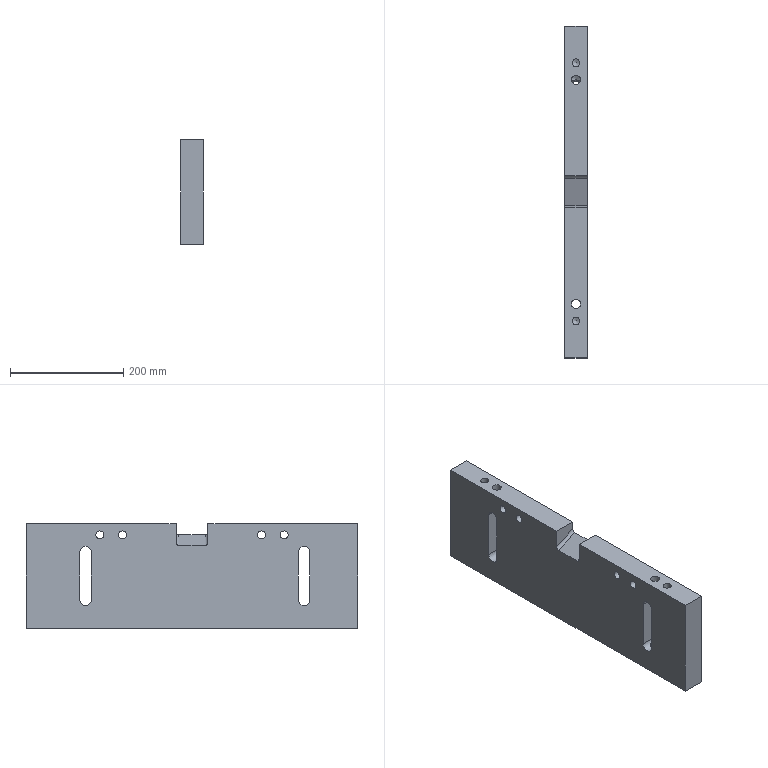Part | STEP file | 1 solid | 39 faces | box 40 x 585 x 185 mm | volume 4012325 mm3 | cylinder 19 | plane 14 | cone 6 | commonest cylinder face diameters 14 x9 16 x4 20 x4 10 x2
STEP:
#1=CARTESIAN_POINT('',(350.,-207.5,-242.));
#2=VERTEX_POINT('',#1);
#3=CARTESIAN_POINT('',(350.,-187.5,-242.));
#4=VERTEX_POINT('',#3);
#5=CARTESIAN_POINT('',(350.,-197.5,-242.));
#6=DIRECTION('',(1.,0.,0.));
#7=DIRECTION('',(0.,0.,-1.));
#8=AXIS2_PLACEMENT_3D('',#5,#6,#7);
#9=CIRCLE('',#8,10.);
#10=EDGE_CURVE('',#2,#4,#9,.T.);
#11=ORIENTED_EDGE('',*,*,#10,.F.);
#12=CARTESIAN_POINT('',(350.,-207.5,-157.));
#13=VERTEX_POINT('',#12);
#14=CARTESIAN_POINT('',(350.,-207.5,-292.));
#15=DIRECTION('',(0.,0.,1.));
#16=VECTOR('',#15,1.);
#17=LINE('',#14,#16);
#18=EDGE_CURVE('',#2,#13,#17,.T.);
#19=ORIENTED_EDGE('',*,*,#18,.T.);
#20=CARTESIAN_POINT('',(350.,-187.5,-157.));
#21=VERTEX_POINT('',#20);
#22=CARTESIAN_POINT('',(350.,-197.5,-157.));
#23=DIRECTION('',(1.,0.,0.));
#24=DIRECTION('',(0.,0.,-1.));
#25=AXIS2_PLACEMENT_3D('',#22,#23,#24);
#26=CIRCLE('',#25,10.);
#27=EDGE_CURVE('',#21,#13,#26,.T.);
#28=ORIENTED_EDGE('',*,*,#27,.F.);
#29=CARTESIAN_POINT('',(350.,-187.5,-107.));
#30=DIRECTION('',(0.,0.,1.));
#31=VECTOR('',#30,1.);
#32=LINE('',#29,#31);
#33=EDGE_CURVE('',#4,#21,#32,.T.);
#34=ORIENTED_EDGE('',*,*,#33,.F.);
#35=EDGE_LOOP('',(#11,#19,#28,#34));
#36=FACE_BOUND('',#35,.T.);
#37=CARTESIAN_POINT('',(350.,28.14,-121.483));
#38=VERTEX_POINT('',#37);
#39=CARTESIAN_POINT('',(350.,28.14,-107.));
#40=VERTEX_POINT('',#39);
#41=CARTESIAN_POINT('',(350.,28.14,-107.));
#42=DIRECTION('',(0.,0.,1.));
#43=VECTOR('',#42,1.);
#44=LINE('',#41,#43);
#45=EDGE_CURVE('',#38,#40,#44,.T.);
#46=ORIENTED_EDGE('',*,*,#45,.F.);
#47=CARTESIAN_POINT('',(350.,23.14,-127.));
#48=VERTEX_POINT('',#47);
#49=CARTESIAN_POINT('',(350.,23.14,-121.483));
#50=DIRECTION('',(-1.,0.,0.));
#51=DIRECTION('',(0.,0.,-1.));
#52=AXIS2_PLACEMENT_3D('',#49,#50,#51);
#53=ELLIPSE('',#52,5.517,5.);
#54=EDGE_CURVE('',#38,#48,#53,.T.);
#55=ORIENTED_EDGE('',*,*,#54,.T.);
#56=CARTESIAN_POINT('',(350.,-23.14,-127.));
#57=VERTEX_POINT('',#56);
#58=CARTESIAN_POINT('',(350.,-1.,-127.));
#59=DIRECTION('',(0.,1.,0.));
#60=VECTOR('',#59,1.);
#61=LINE('',#58,#60);
#62=EDGE_CURVE('',#57,#48,#61,.T.);
#63=ORIENTED_EDGE('',*,*,#62,.F.);
#64=CARTESIAN_POINT('',(350.,-28.14,-121.483));
#65=VERTEX_POINT('',#64);
#66=CARTESIAN_POINT('',(350.,-23.14,-121.483));
#67=DIRECTION('',(-1.,0.,0.));
#68=DIRECTION('',(0.,0.,1.));
#69=AXIS2_PLACEMENT_3D('',#66,#67,#68);
#70=ELLIPSE('',#69,5.517,5.);
#71=EDGE_CURVE('',#57,#65,#70,.T.);
#72=ORIENTED_EDGE('',*,*,#71,.T.);
#73=CARTESIAN_POINT('',(350.,-28.14,-107.));
#74=VERTEX_POINT('',#73);
#75=CARTESIAN_POINT('',(350.,-28.14,-107.));
#76=DIRECTION('',(0.,0.,1.));
#77=VECTOR('',#76,1.);
#78=LINE('',#75,#77);
#79=EDGE_CURVE('',#65,#74,#78,.T.);
#80=ORIENTED_EDGE('',*,*,#79,.T.);
#81=CARTESIAN_POINT('',(350.,-292.5,-107.));
#82=VERTEX_POINT('',#81);
#83=CARTESIAN_POINT('',(350.,-1.,-107.));
#84=DIRECTION('',(0.,-1.,0.));
#85=VECTOR('',#84,1.);
#86=LINE('',#83,#85);
#87=EDGE_CURVE('',#74,#82,#86,.T.);
#88=ORIENTED_EDGE('',*,*,#87,.T.);
#89=CARTESIAN_POINT('',(350.,-292.5,-292.));
#90=VERTEX_POINT('',#89);
#91=CARTESIAN_POINT('',(350.,-292.5,-107.));
#92=DIRECTION('',(0.,0.,1.));
#93=VECTOR('',#92,1.);
#94=LINE('',#91,#93);
#95=EDGE_CURVE('',#90,#82,#94,.T.);
#96=ORIENTED_EDGE('',*,*,#95,.F.);
#97=CARTESIAN_POINT('',(350.,292.5,-292.));
#98=VERTEX_POINT('',#97);
#99=CARTESIAN_POINT('',(350.,-1.,-292.));
#100=DIRECTION('',(0.,-1.,0.));
#101=VECTOR('',#100,1.);
#102=LINE('',#99,#101);
#103=EDGE_CURVE('',#98,#90,#102,.T.);
#104=ORIENTED_EDGE('',*,*,#103,.F.);
#105=CARTESIAN_POINT('',(350.,292.5,-107.));
#106=VERTEX_POINT('',#105);
#107=CARTESIAN_POINT('',(350.,292.5,-107.));
#108=DIRECTION('',(0.,0.,1.));
#109=VECTOR('',#108,1.);
#110=LINE('',#107,#109);
#111=EDGE_CURVE('',#98,#106,#110,.T.);
#112=ORIENTED_EDGE('',*,*,#111,.T.);
#113=CARTESIAN_POINT('',(350.,-1.,-107.));
#114=DIRECTION('',(0.,-1.,0.));
#115=VECTOR('',#114,1.);
#116=LINE('',#113,#115);
#117=EDGE_CURVE('',#106,#40,#116,.T.);
#118=ORIENTED_EDGE('',*,*,#117,.T.);
#119=EDGE_LOOP('',(#46,#55,#63,#72,#80,#88,#96,#104,#112,#118));
#120=FACE_BOUND('',#119,.T.);
#121=CARTESIAN_POINT('',(350.,-162.5,-120.));
#122=VERTEX_POINT('',#121);
#123=CARTESIAN_POINT('',(350.,-162.5,-127.));
#124=DIRECTION('',(-1.,0.,0.));
#125=DIRECTION('',(0.,0.,1.));
#126=AXIS2_PLACEMENT_3D('',#123,#124,#125);
#127=CIRCLE('',#126,7.);
#128=EDGE_CURVE('',#122,#122,#127,.T.);
#129=ORIENTED_EDGE('',*,*,#128,.T.);
#130=EDGE_LOOP('',(#129));
#131=FACE_BOUND('',#130,.T.);
#132=CARTESIAN_POINT('',(350.,-122.5,-120.));
#133=VERTEX_POINT('',#132);
#134=CARTESIAN_POINT('',(350.,-122.5,-127.));
#135=DIRECTION('',(1.,0.,0.));
#136=DIRECTION('',(0.,0.,1.));
#137=AXIS2_PLACEMENT_3D('',#134,#135,#136);
#138=CIRCLE('',#137,7.);
#139=EDGE_CURVE('',#133,#133,#138,.T.);
#140=ORIENTED_EDGE('',*,*,#139,.F.);
#141=EDGE_LOOP('',(#140));
#142=FACE_BOUND('',#141,.T.);
#143=CARTESIAN_POINT('',(350.,162.5,-120.));
#144=VERTEX_POINT('',#143);
#145=CARTESIAN_POINT('',(350.,162.5,-127.));
#146=DIRECTION('',(1.,0.,0.));
#147=DIRECTION('',(0.,0.,1.));
#148=AXIS2_PLACEMENT_3D('',#145,#146,#147);
#149=CIRCLE('',#148,7.);
#150=EDGE_CURVE('',#144,#144,#149,.T.);
#151=ORIENTED_EDGE('',*,*,#150,.F.);
#152=EDGE_LOOP('',(#151));
#153=FACE_BOUND('',#152,.T.);
#154=CARTESIAN_POINT('',(350.,122.5,-120.));
#155=VERTEX_POINT('',#154);
#156=CARTESIAN_POINT('',(350.,122.5,-127.));
#157=DIRECTION('',(-1.,0.,0.));
#158=DIRECTION('',(0.,0.,1.));
#159=AXIS2_PLACEMENT_3D('',#156,#157,#158);
#160=CIRCLE('',#159,7.);
#161=EDGE_CURVE('',#155,#155,#160,.T.);
#162=ORIENTED_EDGE('',*,*,#161,.T.);
#163=EDGE_LOOP('',(#162));
#164=FACE_BOUND('',#163,.T.);
#165=CARTESIAN_POINT('',(350.,177.5,-242.));
#166=VERTEX_POINT('',#165);
#167=CARTESIAN_POINT('',(350.,197.5,-242.));
#168=VERTEX_POINT('',#167);
#169=CARTESIAN_POINT('',(350.,187.5,-242.));
#170=DIRECTION('',(1.,0.,0.));
#171=DIRECTION('',(0.,0.,-1.));
#172=AXIS2_PLACEMENT_3D('',#169,#170,#171);
#173=CIRCLE('',#172,10.);
#174=EDGE_CURVE('',#166,#168,#173,.T.);
#175=ORIENTED_EDGE('',*,*,#174,.F.);
#176=CARTESIAN_POINT('',(350.,177.5,-157.));
#177=VERTEX_POINT('',#176);
#178=CARTESIAN_POINT('',(350.,177.5,-292.));
#179=DIRECTION('',(0.,0.,1.));
#180=VECTOR('',#179,1.);
#181=LINE('',#178,#180);
#182=EDGE_CURVE('',#166,#177,#181,.T.);
#183=ORIENTED_EDGE('',*,*,#182,.T.);
#184=CARTESIAN_POINT('',(350.,197.5,-157.));
#185=VERTEX_POINT('',#184);
#186=CARTESIAN_POINT('',(350.,187.5,-157.));
#187=DIRECTION('',(1.,0.,0.));
#188=DIRECTION('',(0.,0.,-1.));
#189=AXIS2_PLACEMENT_3D('',#186,#187,#188);
#190=CIRCLE('',#189,10.);
#191=EDGE_CURVE('',#185,#177,#190,.T.);
#192=ORIENTED_EDGE('',*,*,#191,.F.);
#193=CARTESIAN_POINT('',(350.,197.5,-107.));
#194=DIRECTION('',(0.,0.,1.));
#195=VECTOR('',#194,1.);
#196=LINE('',#193,#195);
#197=EDGE_CURVE('',#168,#185,#196,.T.);
#198=ORIENTED_EDGE('',*,*,#197,.F.);
#199=EDGE_LOOP('',(#175,#183,#192,#198));
#200=FACE_BOUND('',#199,.T.);
#201=CARTESIAN_POINT('',(350.,-1.,-107.));
#202=DIRECTION('',(1.,0.,0.));
#203=DIRECTION('',(0.,-1.,0.));
#204=AXIS2_PLACEMENT_3D('',#201,#202,#203);
#205=PLANE('',#204);
#206=ADVANCED_FACE('',(#36,#120,#131,#142,#153,#164,#200),#205,.T.);
#207=CARTESIAN_POINT('',(310.,-187.5,-242.));
#208=VERTEX_POINT('',#207);
#209=CARTESIAN_POINT('',(310.,-207.5,-242.));
#210=VERTEX_POINT('',#209);
#211=CARTESIAN_POINT('',(310.,-197.5,-242.));
#212=DIRECTION('',(-1.,0.,0.));
#213=DIRECTION('',(0.,0.,1.));
#214=AXIS2_PLACEMENT_3D('',#211,#212,#213);
#215=CIRCLE('',#214,10.);
#216=EDGE_CURVE('',#208,#210,#215,.T.);
#217=ORIENTED_EDGE('',*,*,#216,.F.);
#218=CARTESIAN_POINT('',(310.,-187.5,-157.));
#219=VERTEX_POINT('',#218);
#220=CARTESIAN_POINT('',(310.,-187.5,-292.));
#221=DIRECTION('',(0.,0.,1.));
#222=VECTOR('',#221,1.);
#223=LINE('',#220,#222);
#224=EDGE_CURVE('',#208,#219,#223,.T.);
#225=ORIENTED_EDGE('',*,*,#224,.T.);
#226=CARTESIAN_POINT('',(310.,-207.5,-157.));
#227=VERTEX_POINT('',#226);
#228=CARTESIAN_POINT('',(310.,-197.5,-157.));
#229=DIRECTION('',(-1.,0.,0.));
#230=DIRECTION('',(0.,0.,1.));
#231=AXIS2_PLACEMENT_3D('',#228,#229,#230);
#232=CIRCLE('',#231,10.);
#233=EDGE_CURVE('',#227,#219,#232,.T.);
#234=ORIENTED_EDGE('',*,*,#233,.F.);
#235=CARTESIAN_POINT('',(310.,-207.5,-107.));
#236=DIRECTION('',(0.,0.,1.));
#237=VECTOR('',#236,1.);
#238=LINE('',#235,#237);
#239=EDGE_CURVE('',#210,#227,#238,.T.);
#240=ORIENTED_EDGE('',*,*,#239,.F.);
#241=EDGE_LOOP('',(#217,#225,#234,#240));
#242=FACE_BOUND('',#241,.T.);
#243=CARTESIAN_POINT('',(310.,122.5,-120.));
#244=VERTEX_POINT('',#243);
#245=CARTESIAN_POINT('',(310.,122.5,-127.));
#246=DIRECTION('',(-1.,0.,0.));
#247=DIRECTION('',(0.,0.,1.));
#248=AXIS2_PLACEMENT_3D('',#245,#246,#247);
#249=CIRCLE('',#248,7.);
#250=EDGE_CURVE('',#244,#244,#249,.T.);
#251=ORIENTED_EDGE('',*,*,#250,.F.);
#252=EDGE_LOOP('',(#251));
#253=FACE_BOUND('',#252,.T.);
#254=CARTESIAN_POINT('',(310.,162.5,-120.));
#255=VERTEX_POINT('',#254);
#256=CARTESIAN_POINT('',(310.,162.5,-127.));
#257=DIRECTION('',(1.,0.,0.));
#258=DIRECTION('',(0.,0.,1.));
#259=AXIS2_PLACEMENT_3D('',#256,#257,#258);
#260=CIRCLE('',#259,7.);
#261=EDGE_CURVE('',#255,#255,#260,.T.);
#262=ORIENTED_EDGE('',*,*,#261,.T.);
#263=EDGE_LOOP('',(#262));
#264=FACE_BOUND('',#263,.T.);
#265=CARTESIAN_POINT('',(310.,-122.5,-120.));
#266=VERTEX_POINT('',#265);
#267=CARTESIAN_POINT('',(310.,-122.5,-127.));
#268=DIRECTION('',(1.,0.,0.));
#269=DIRECTION('',(0.,0.,1.));
#270=AXIS2_PLACEMENT_3D('',#267,#268,#269);
#271=CIRCLE('',#270,7.);
#272=EDGE_CURVE('',#266,#266,#271,.T.);
#273=ORIENTED_EDGE('',*,*,#272,.T.);
#274=EDGE_LOOP('',(#273));
#275=FACE_BOUND('',#274,.T.);
#276=CARTESIAN_POINT('',(310.,-162.5,-120.));
#277=VERTEX_POINT('',#276);
#278=CARTESIAN_POINT('',(310.,-162.5,-127.));
#279=DIRECTION('',(-1.,0.,0.));
#280=DIRECTION('',(0.,0.,1.));
#281=AXIS2_PLACEMENT_3D('',#278,#279,#280);
#282=CIRCLE('',#281,7.);
#283=EDGE_CURVE('',#277,#277,#282,.T.);
#284=ORIENTED_EDGE('',*,*,#283,.F.);
#285=EDGE_LOOP('',(#284));
#286=FACE_BOUND('',#285,.T.);
#287=CARTESIAN_POINT('',(310.,-292.5,-107.));
#288=VERTEX_POINT('',#287);
#289=CARTESIAN_POINT('',(310.,-28.14,-107.));
#290=VERTEX_POINT('',#289);
#291=CARTESIAN_POINT('',(310.,-1.,-107.));
#292=DIRECTION('',(0.,1.,0.));
#293=VECTOR('',#292,1.);
#294=LINE('',#291,#293);
#295=EDGE_CURVE('',#288,#290,#294,.T.);
#296=ORIENTED_EDGE('',*,*,#295,.T.);
#297=CARTESIAN_POINT('',(310.,-28.14,-140.135));
#298=VERTEX_POINT('',#297);
#299=CARTESIAN_POINT('',(310.,-28.14,-107.));
#300=DIRECTION('',(0.,0.,-1.));
#301=VECTOR('',#300,1.);
#302=LINE('',#299,#301);
#303=EDGE_CURVE('',#290,#298,#302,.T.);
#304=ORIENTED_EDGE('',*,*,#303,.T.);
#305=CARTESIAN_POINT('',(310.,-23.14,-145.652));
#306=VERTEX_POINT('',#305);
#307=CARTESIAN_POINT('',(310.,-23.14,-140.135));
#308=DIRECTION('',(1.,0.,0.));
#309=DIRECTION('',(0.,0.,1.));
#310=AXIS2_PLACEMENT_3D('',#307,#308,#309);
#311=ELLIPSE('',#310,5.517,5.);
#312=EDGE_CURVE('',#298,#306,#311,.T.);
#313=ORIENTED_EDGE('',*,*,#312,.T.);
#314=CARTESIAN_POINT('',(310.,23.14,-145.652));
#315=VERTEX_POINT('',#314);
#316=CARTESIAN_POINT('',(310.,-1.,-145.652));
#317=DIRECTION('',(0.,1.,0.));
#318=VECTOR('',#317,1.);
#319=LINE('',#316,#318);
#320=EDGE_CURVE('',#306,#315,#319,.T.);
#321=ORIENTED_EDGE('',*,*,#320,.T.);
#322=CARTESIAN_POINT('',(310.,28.14,-140.135));
#323=VERTEX_POINT('',#322);
#324=CARTESIAN_POINT('',(310.,23.14,-140.135));
#325=DIRECTION('',(1.,0.,0.));
#326=DIRECTION('',(0.,0.,-1.));
#327=AXIS2_PLACEMENT_3D('',#324,#325,#326);
#328=ELLIPSE('',#327,5.517,5.);
#329=EDGE_CURVE('',#315,#323,#328,.T.);
#330=ORIENTED_EDGE('',*,*,#329,.T.);
#331=CARTESIAN_POINT('',(310.,28.14,-107.));
#332=VERTEX_POINT('',#331);
#333=CARTESIAN_POINT('',(310.,28.14,-107.));
#334=DIRECTION('',(0.,0.,1.));
#335=VECTOR('',#334,1.);
#336=LINE('',#333,#335);
#337=EDGE_CURVE('',#323,#332,#336,.T.);
#338=ORIENTED_EDGE('',*,*,#337,.T.);
#339=CARTESIAN_POINT('',(310.,292.5,-107.));
#340=VERTEX_POINT('',#339);
#341=CARTESIAN_POINT('',(310.,-1.,-107.));
#342=DIRECTION('',(0.,1.,0.));
#343=VECTOR('',#342,1.);
#344=LINE('',#341,#343);
#345=EDGE_CURVE('',#332,#340,#344,.T.);
#346=ORIENTED_EDGE('',*,*,#345,.T.);
#347=CARTESIAN_POINT('',(310.,292.5,-292.));
#348=VERTEX_POINT('',#347);
#349=CARTESIAN_POINT('',(310.,292.5,-107.));
#350=DIRECTION('',(0.,0.,1.));
#351=VECTOR('',#350,1.);
#352=LINE('',#349,#351);
#353=EDGE_CURVE('',#348,#340,#352,.T.);
#354=ORIENTED_EDGE('',*,*,#353,.F.);
#355=CARTESIAN_POINT('',(310.,-292.5,-292.));
#356=VERTEX_POINT('',#355);
#357=CARTESIAN_POINT('',(310.,-1.,-292.));
#358=DIRECTION('',(0.,1.,0.));
#359=VECTOR('',#358,1.);
#360=LINE('',#357,#359);
#361=EDGE_CURVE('',#356,#348,#360,.T.);
#362=ORIENTED_EDGE('',*,*,#361,.F.);
#363=CARTESIAN_POINT('',(310.,-292.5,-107.));
#364=DIRECTION('',(0.,0.,1.));
#365=VECTOR('',#364,1.);
#366=LINE('',#363,#365);
#367=EDGE_CURVE('',#356,#288,#366,.T.);
#368=ORIENTED_EDGE('',*,*,#367,.T.);
#369=EDGE_LOOP('',(#296,#304,#313,#321,#330,#338,#346,#354,#362,#368));
#370=FACE_BOUND('',#369,.T.);
#371=CARTESIAN_POINT('',(310.,197.5,-242.));
#372=VERTEX_POINT('',#371);
#373=CARTESIAN_POINT('',(310.,177.5,-242.));
#374=VERTEX_POINT('',#373);
#375=CARTESIAN_POINT('',(310.,187.5,-242.));
#376=DIRECTION('',(-1.,0.,0.));
#377=DIRECTION('',(0.,0.,1.));
#378=AXIS2_PLACEMENT_3D('',#375,#376,#377);
#379=CIRCLE('',#378,10.);
#380=EDGE_CURVE('',#372,#374,#379,.T.);
#381=ORIENTED_EDGE('',*,*,#380,.F.);
#382=CARTESIAN_POINT('',(310.,197.5,-157.));
#383=VERTEX_POINT('',#382);
#384=CARTESIAN_POINT('',(310.,197.5,-292.));
#385=DIRECTION('',(0.,0.,1.));
#386=VECTOR('',#385,1.);
#387=LINE('',#384,#386);
#388=EDGE_CURVE('',#372,#383,#387,.T.);
#389=ORIENTED_EDGE('',*,*,#388,.T.);
#390=CARTESIAN_POINT('',(310.,177.5,-157.));
#391=VERTEX_POINT('',#390);
#392=CARTESIAN_POINT('',(310.,187.5,-157.));
#393=DIRECTION('',(-1.,0.,0.));
#394=DIRECTION('',(0.,0.,1.));
#395=AXIS2_PLACEMENT_3D('',#392,#393,#394);
#396=CIRCLE('',#395,10.);
#397=EDGE_CURVE('',#391,#383,#396,.T.);
#398=ORIENTED_EDGE('',*,*,#397,.F.);
#399=CARTESIAN_POINT('',(310.,177.5,-107.));
#400=DIRECTION('',(0.,0.,1.));
#401=VECTOR('',#400,1.);
#402=LINE('',#399,#401);
#403=EDGE_CURVE('',#374,#391,#402,.T.);
#404=ORIENTED_EDGE('',*,*,#403,.F.);
#405=EDGE_LOOP('',(#381,#389,#398,#404));
#406=FACE_BOUND('',#405,.T.);
#407=CARTESIAN_POINT('',(310.,-1.,-107.));
#408=DIRECTION('',(-1.,0.,0.));
#409=DIRECTION('',(0.,1.,0.));
#410=AXIS2_PLACEMENT_3D('',#407,#408,#409);
#411=PLANE('',#410);
#412=ADVANCED_FACE('',(#242,#253,#264,#275,#286,#370,#406),#411,.T.);
#413=CARTESIAN_POINT('',(338.,-197.5,-107.));
#414=VERTEX_POINT('',#413);
#415=CARTESIAN_POINT('',(330.,-197.5,-107.));
#416=DIRECTION('',(0.,0.,1.));
#417=DIRECTION('',(1.,0.,0.));
#418=AXIS2_PLACEMENT_3D('',#415,#416,#417);
#419=CIRCLE('',#418,8.);
#420=EDGE_CURVE('',#414,#414,#419,.T.);
#421=ORIENTED_EDGE('',*,*,#420,.F.);
#422=EDGE_LOOP('',(#421));
#423=FACE_BOUND('',#422,.T.);
#424=CARTESIAN_POINT('',(-108.5,-28.14,-107.));
#425=DIRECTION('',(1.,0.,0.));
#426=VECTOR('',#425,1.);
#427=LINE('',#424,#426);
#428=EDGE_CURVE('',#290,#74,#427,.T.);
#429=ORIENTED_EDGE('',*,*,#428,.F.);
#430=ORIENTED_EDGE('',*,*,#295,.F.);
#431=CARTESIAN_POINT('',(-108.5,-292.5,-107.));
#432=DIRECTION('',(-1.,0.,0.));
#433=VECTOR('',#432,1.);
#434=LINE('',#431,#433);
#435=EDGE_CURVE('',#82,#288,#434,.T.);
#436=ORIENTED_EDGE('',*,*,#435,.F.);
#437=ORIENTED_EDGE('',*,*,#87,.F.);
#438=EDGE_LOOP('',(#429,#430,#436,#437));
#439=FACE_BOUND('',#438,.T.);
#440=CARTESIAN_POINT('',(323.,-227.5,-107.));
#441=VERTEX_POINT('',#440);
#442=CARTESIAN_POINT('',(330.,-227.5,-107.));
#443=DIRECTION('',(0.,0.,-1.));
#444=DIRECTION('',(-1.,0.,0.));
#445=AXIS2_PLACEMENT_3D('',#442,#443,#444);
#446=CIRCLE('',#445,7.);
#447=EDGE_CURVE('',#441,#441,#446,.T.);
#448=ORIENTED_EDGE('',*,*,#447,.T.);
#449=EDGE_LOOP('',(#448));
#450=FACE_BOUND('',#449,.T.);
#451=CARTESIAN_POINT('',(-108.5,-1.,-107.));
#452=DIRECTION('',(0.,0.,1.));
#453=DIRECTION('',(-1.,0.,0.));
#454=AXIS2_PLACEMENT_3D('',#451,#452,#453);
#455=PLANE('',#454);
#456=ADVANCED_FACE('',(#423,#439,#450),#455,.T.);
#457=ORIENTED_EDGE('',*,*,#111,.F.);
#458=CARTESIAN_POINT('',(-108.5,292.5,-292.));
#459=DIRECTION('',(1.,0.,0.));
#460=VECTOR('',#459,1.);
#461=LINE('',#458,#460);
#462=EDGE_CURVE('',#348,#98,#461,.T.);
#463=ORIENTED_EDGE('',*,*,#462,.F.);
#464=ORIENTED_EDGE('',*,*,#353,.T.);
#465=CARTESIAN_POINT('',(-108.5,292.5,-107.));
#466=DIRECTION('',(1.,0.,0.));
#467=VECTOR('',#466,1.);
#468=LINE('',#465,#467);
#469=EDGE_CURVE('',#340,#106,#468,.T.);
#470=ORIENTED_EDGE('',*,*,#469,.T.);
#471=EDGE_LOOP('',(#457,#463,#464,#470));
#472=FACE_OUTER_BOUND('',#471,.T.);
#473=CARTESIAN_POINT('',(-108.5,292.5,-107.));
#474=DIRECTION('',(0.,1.,0.));
#475=DIRECTION('',(1.,0.,0.));
#476=AXIS2_PLACEMENT_3D('',#473,#474,#475);
#477=PLANE('',#476);
#478=ADVANCED_FACE('',(#472),#477,.T.);
#479=CARTESIAN_POINT('',(-108.5,-292.5,-292.));
#480=DIRECTION('',(-1.,0.,0.));
#481=VECTOR('',#480,1.);
#482=LINE('',#479,#481);
#483=EDGE_CURVE('',#90,#356,#482,.T.);
#484=ORIENTED_EDGE('',*,*,#483,.F.);
#485=ORIENTED_EDGE('',*,*,#95,.T.);
#486=ORIENTED_EDGE('',*,*,#435,.T.);
#487=ORIENTED_EDGE('',*,*,#367,.F.);
#488=EDGE_LOOP('',(#484,#485,#486,#487));
#489=FACE_OUTER_BOUND('',#488,.T.);
#490=CARTESIAN_POINT('',(-108.5,-292.5,-107.));
#491=DIRECTION('',(0.,-1.,0.));
#492=DIRECTION('',(-1.,0.,0.));
#493=AXIS2_PLACEMENT_3D('',#490,#491,#492);
#494=PLANE('',#493);
#495=ADVANCED_FACE('',(#489),#494,.T.);
#496=CARTESIAN_POINT('',(338.,197.5,-107.));
#497=VERTEX_POINT('',#496);
#498=CARTESIAN_POINT('',(330.,197.5,-107.));
#499=DIRECTION('',(0.,0.,-1.));
#500=DIRECTION('',(1.,0.,0.));
#501=AXIS2_PLACEMENT_3D('',#498,#499,#500);
#502=CIRCLE('',#501,8.);
#503=EDGE_CURVE('',#497,#497,#502,.T.);
#504=ORIENTED_EDGE('',*,*,#503,.T.);
#505=EDGE_LOOP('',(#504));
#506=FACE_BOUND('',#505,.T.);
#507=CARTESIAN_POINT('',(-108.5,28.14,-107.));
#508=DIRECTION('',(-1.,0.,0.));
#509=VECTOR('',#508,1.);
#510=LINE('',#507,#509);
#511=EDGE_CURVE('',#40,#332,#510,.T.);
#512=ORIENTED_EDGE('',*,*,#511,.F.);
#513=ORIENTED_EDGE('',*,*,#117,.F.);
#514=ORIENTED_EDGE('',*,*,#469,.F.);
#515=ORIENTED_EDGE('',*,*,#345,.F.);
#516=EDGE_LOOP('',(#512,#513,#514,#515));
#517=FACE_BOUND('',#516,.T.);
#518=CARTESIAN_POINT('',(323.,227.5,-107.));
#519=VERTEX_POINT('',#518);
#520=CARTESIAN_POINT('',(330.,227.5,-107.));
#521=DIRECTION('',(0.,0.,1.));
#522=DIRECTION('',(-1.,0.,0.));
#523=AXIS2_PLACEMENT_3D('',#520,#521,#522);
#524=CIRCLE('',#523,7.);
#525=EDGE_CURVE('',#519,#519,#524,.T.);
#526=ORIENTED_EDGE('',*,*,#525,.F.);
#527=EDGE_LOOP('',(#526));
#528=FACE_BOUND('',#527,.T.);
#529=CARTESIAN_POINT('',(-108.5,-1.,-107.));
#530=DIRECTION('',(0.,0.,1.));
#531=DIRECTION('',(-1.,0.,0.));
#532=AXIS2_PLACEMENT_3D('',#529,#530,#531);
#533=PLANE('',#532);
#534=ADVANCED_FACE('',(#506,#517,#528),#533,.T.);
#535=CARTESIAN_POINT('',(338.,187.5,-292.));
#536=VERTEX_POINT('',#535);
#537=CARTESIAN_POINT('',(330.,187.5,-292.));
#538=DIRECTION('',(0.,0.,1.));
#539=DIRECTION('',(1.,0.,0.));
#540=AXIS2_PLACEMENT_3D('',#537,#538,#539);
#541=CIRCLE('',#540,8.);
#542=EDGE_CURVE('',#536,#536,#541,.T.);
#543=ORIENTED_EDGE('',*,*,#542,.T.);
#544=EDGE_LOOP('',(#543));
#545=FACE_BOUND('',#544,.T.);
#546=CARTESIAN_POINT('',(338.,-197.5,-292.));
#547=VERTEX_POINT('',#546);
#548=CARTESIAN_POINT('',(330.,-197.5,-292.));
#549=DIRECTION('',(0.,0.,-1.));
#550=DIRECTION('',(1.,0.,0.));
#551=AXIS2_PLACEMENT_3D('',#548,#549,#550);
#552=CIRCLE('',#551,8.);
#553=EDGE_CURVE('',#547,#547,#552,.T.);
#554=ORIENTED_EDGE('',*,*,#553,.F.);
#555=EDGE_LOOP('',(#554));
#556=FACE_BOUND('',#555,.T.);
#557=ORIENTED_EDGE('',*,*,#361,.T.);
#558=ORIENTED_EDGE('',*,*,#462,.T.);
#559=ORIENTED_EDGE('',*,*,#103,.T.);
#560=ORIENTED_EDGE('',*,*,#483,.T.);
#561=EDGE_LOOP('',(#557,#558,#559,#560));
#562=FACE_BOUND('',#561,.T.);
#563=CARTESIAN_POINT('',(337.,267.5,-292.));
#564=VERTEX_POINT('',#563);
#565=CARTESIAN_POINT('',(330.,267.5,-292.));
#566=DIRECTION('',(0.,0.,1.));
#567=DIRECTION('',(1.,0.,0.));
#568=AXIS2_PLACEMENT_3D('',#565,#566,#567);
#569=CIRCLE('',#568,7.);
#570=EDGE_CURVE('',#564,#564,#569,.T.);
#571=ORIENTED_EDGE('',*,*,#570,.T.);
#572=EDGE_LOOP('',(#571));
#573=FACE_BOUND('',#572,.T.);
#574=CARTESIAN_POINT('',(337.,-267.5,-292.));
#575=VERTEX_POINT('',#574);
#576=CARTESIAN_POINT('',(330.,-267.5,-292.));
#577=DIRECTION('',(0.,0.,-1.));
#578=DIRECTION('',(1.,0.,0.));
#579=AXIS2_PLACEMENT_3D('',#576,#577,#578);
#580=CIRCLE('',#579,7.);
#581=EDGE_CURVE('',#575,#575,#580,.T.);
#582=ORIENTED_EDGE('',*,*,#581,.F.);
#583=EDGE_LOOP('',(#582));
#584=FACE_BOUND('',#583,.T.);
#585=CARTESIAN_POINT('',(337.,0.,-292.));
#586=VERTEX_POINT('',#585);
#587=CARTESIAN_POINT('',(330.,0.,-292.));
#588=DIRECTION('',(0.,0.,1.));
#589=DIRECTION('',(1.,0.,0.));
#590=AXIS2_PLACEMENT_3D('',#587,#588,#589);
#591=CIRCLE('',#590,7.);
#592=EDGE_CURVE('',#586,#586,#591,.T.);
#593=ORIENTED_EDGE('',*,*,#592,.T.);
#594=EDGE_LOOP('',(#593));
#595=FACE_BOUND('',#594,.T.);
#596=CARTESIAN_POINT('',(-98.5,-1.,-292.));
#597=DIRECTION('',(0.,0.,-1.));
#598=DIRECTION('',(-1.,0.,0.));
#599=AXIS2_PLACEMENT_3D('',#596,#597,#598);
#600=PLANE('',#599);
#601=ADVANCED_FACE('',(#545,#556,#562,#573,#584,#595),#600,.T.);
#602=ORIENTED_EDGE('',*,*,#62,.T.);
#603=CARTESIAN_POINT('',(310.,23.14,-145.652));
#604=DIRECTION('',(-0.9063,0.,-0.4226));
#605=VECTOR('',#604,1.);
#606=LINE('',#603,#605);
#607=EDGE_CURVE('',#48,#315,#606,.T.);
#608=ORIENTED_EDGE('',*,*,#607,.T.);
#609=ORIENTED_EDGE('',*,*,#320,.F.);
#610=CARTESIAN_POINT('',(350.,-23.14,-127.));
#611=DIRECTION('',(0.9063,0.,0.4226));
#612=VECTOR('',#611,1.);
#613=LINE('',#610,#612);
#614=EDGE_CURVE('',#306,#57,#613,.T.);
#615=ORIENTED_EDGE('',*,*,#614,.T.);
#616=EDGE_LOOP('',(#602,#608,#609,#615));
#617=FACE_OUTER_BOUND('',#616,.T.);
#618=CARTESIAN_POINT('',(324.85,0.,-138.728));
#619=DIRECTION('',(0.4226,0.,-0.9063));
#620=DIRECTION('',(-0.9063,0.,-0.4226));
#621=AXIS2_PLACEMENT_3D('',#618,#619,#620);
#622=PLANE('',#621);
#623=ADVANCED_FACE('',(#617),#622,.F.);
#624=ORIENTED_EDGE('',*,*,#79,.F.);
#625=CARTESIAN_POINT('',(307.887,-28.14,-141.121));
#626=DIRECTION('',(-0.9063,0.,-0.4226));
#627=VECTOR('',#626,1.);
#628=LINE('',#625,#627);
#629=EDGE_CURVE('',#65,#298,#628,.T.);
#630=ORIENTED_EDGE('',*,*,#629,.T.);
#631=ORIENTED_EDGE('',*,*,#303,.F.);
#632=ORIENTED_EDGE('',*,*,#428,.T.);
#633=EDGE_LOOP('',(#624,#630,#631,#632));
#634=FACE_OUTER_BOUND('',#633,.T.);
#635=CARTESIAN_POINT('',(322.25,-28.14,-107.));
#636=DIRECTION('',(0.,-1.,0.));
#637=DIRECTION('',(0.,0.,-1.));
#638=AXIS2_PLACEMENT_3D('',#635,#636,#637);
#639=PLANE('',#638);
#640=ADVANCED_FACE('',(#634),#639,.F.);
#641=ORIENTED_EDGE('',*,*,#337,.F.);
#642=CARTESIAN_POINT('',(347.887,28.14,-122.468));
#643=DIRECTION('',(0.9063,0.,0.4226));
#644=VECTOR('',#643,1.);
#645=LINE('',#642,#644);
#646=EDGE_CURVE('',#323,#38,#645,.T.);
#647=ORIENTED_EDGE('',*,*,#646,.T.);
#648=ORIENTED_EDGE('',*,*,#45,.T.);
#649=ORIENTED_EDGE('',*,*,#511,.T.);
#650=EDGE_LOOP('',(#641,#647,#648,#649));
#651=FACE_OUTER_BOUND('',#650,.T.);
#652=CARTESIAN_POINT('',(322.25,28.14,-107.));
#653=DIRECTION('',(0.,1.,0.));
#654=DIRECTION('',(0.,0.,1.));
#655=AXIS2_PLACEMENT_3D('',#652,#653,#654);
#656=PLANE('',#655);
#657=ADVANCED_FACE('',(#651),#656,.F.);
#658=ORIENTED_EDGE('',*,*,#329,.F.);
#659=ORIENTED_EDGE('',*,*,#607,.F.);
#660=ORIENTED_EDGE('',*,*,#54,.F.);
#661=ORIENTED_EDGE('',*,*,#646,.F.);
#662=EDGE_LOOP('',(#658,#659,#660,#661));
#663=FACE_OUTER_BOUND('',#662,.T.);
#664=CARTESIAN_POINT('',(332.754,23.14,-129.525));
#665=DIRECTION('',(-0.9063,0.,-0.4226));
#666=DIRECTION('',(-0.4226,0.,0.9063));
#667=AXIS2_PLACEMENT_3D('',#664,#665,#666);
#668=CYLINDRICAL_SURFACE('',#667,5.);
#669=ADVANCED_FACE('',(#663),#668,.F.);
#670=ORIENTED_EDGE('',*,*,#71,.F.);
#671=ORIENTED_EDGE('',*,*,#614,.F.);
#672=ORIENTED_EDGE('',*,*,#312,.F.);
#673=ORIENTED_EDGE('',*,*,#629,.F.);
#674=EDGE_LOOP('',(#670,#671,#672,#673));
#675=FACE_OUTER_BOUND('',#674,.T.);
#676=CARTESIAN_POINT('',(332.754,-23.14,-129.525));
#677=DIRECTION('',(0.9063,0.,0.4226));
#678=DIRECTION('',(0.4226,0.,-0.9063));
#679=AXIS2_PLACEMENT_3D('',#676,#677,#678);
#680=CYLINDRICAL_SURFACE('',#679,5.);
#681=ADVANCED_FACE('',(#675),#680,.F.);
#682=CARTESIAN_POINT('',(337.,-227.5,-147.));
#683=VERTEX_POINT('',#682);
#684=CARTESIAN_POINT('',(330.,-227.5,-147.));
#685=DIRECTION('',(0.,0.,1.));
#686=DIRECTION('',(1.,0.,0.));
#687=AXIS2_PLACEMENT_3D('',#684,#685,#686);
#688=CIRCLE('',#687,7.);
#689=EDGE_CURVE('',#683,#683,#688,.T.);
#690=ORIENTED_EDGE('',*,*,#689,.F.);
#691=EDGE_LOOP('',(#690));
#692=FACE_BOUND('',#691,.T.);
#693=ORIENTED_EDGE('',*,*,#447,.F.);
#694=EDGE_LOOP('',(#693));
#695=FACE_BOUND('',#694,.T.);
#696=CARTESIAN_POINT('',(330.,-227.5,-107.));
#697=DIRECTION('',(0.,0.,-1.));
#698=DIRECTION('',(1.,0.,0.));
#699=AXIS2_PLACEMENT_3D('',#696,#697,#698);
#700=CYLINDRICAL_SURFACE('',#699,7.);
#701=ADVANCED_FACE('',(#692,#695),#700,.F.);
#702=ORIENTED_EDGE('',*,*,#689,.T.);
#703=EDGE_LOOP('',(#702));
#704=FACE_BOUND('',#703,.T.);
#705=CARTESIAN_POINT('',(330.,-227.5,-150.));
#706=VERTEX_POINT('',#705);
#707=VERTEX_LOOP('',#706);
#708=FACE_BOUND('',#707,.T.);
#709=CARTESIAN_POINT('',(330.,-227.5,-150.));
#710=DIRECTION('',(0.,0.,1.));
#711=DIRECTION('',(1.,0.,0.));
#712=AXIS2_PLACEMENT_3D('',#709,#710,#711);
#713=CONICAL_SURFACE('',#712,0.,66.801);
#714=ADVANCED_FACE('',(#704,#708),#713,.F.);
#715=CARTESIAN_POINT('',(337.,227.5,-147.));
#716=VERTEX_POINT('',#715);
#717=CARTESIAN_POINT('',(330.,227.5,-147.));
#718=DIRECTION('',(0.,0.,-1.));
#719=DIRECTION('',(1.,0.,0.));
#720=AXIS2_PLACEMENT_3D('',#717,#718,#719);
#721=CIRCLE('',#720,7.);
#722=EDGE_CURVE('',#716,#716,#721,.T.);
#723=ORIENTED_EDGE('',*,*,#722,.T.);
#724=EDGE_LOOP('',(#723));
#725=FACE_BOUND('',#724,.T.);
#726=ORIENTED_EDGE('',*,*,#525,.T.);
#727=EDGE_LOOP('',(#726));
#728=FACE_BOUND('',#727,.T.);
#729=CARTESIAN_POINT('',(330.,227.5,-107.));
#730=DIRECTION('',(0.,0.,-1.));
#731=DIRECTION('',(1.,0.,0.));
#732=AXIS2_PLACEMENT_3D('',#729,#730,#731);
#733=CYLINDRICAL_SURFACE('',#732,7.);
#734=ADVANCED_FACE('',(#725,#728),#733,.F.);
#735=ORIENTED_EDGE('',*,*,#722,.F.);
#736=EDGE_LOOP('',(#735));
#737=FACE_BOUND('',#736,.T.);
#738=CARTESIAN_POINT('',(330.,227.5,-150.));
#739=VERTEX_POINT('',#738);
#740=VERTEX_LOOP('',#739);
#741=FACE_BOUND('',#740,.T.);
#742=CARTESIAN_POINT('',(330.,227.5,-150.));
#743=DIRECTION('',(0.,0.,1.));
#744=DIRECTION('',(1.,0.,0.));
#745=AXIS2_PLACEMENT_3D('',#742,#743,#744);
#746=CONICAL_SURFACE('',#745,0.,66.801);
#747=ADVANCED_FACE('',(#737,#741),#746,.F.);
#748=CARTESIAN_POINT('',(323.,267.5,-252.));
#749=VERTEX_POINT('',#748);
#750=CARTESIAN_POINT('',(330.,267.5,-252.));
#751=DIRECTION('',(0.,0.,-1.));
#752=DIRECTION('',(-1.,0.,0.));
#753=AXIS2_PLACEMENT_3D('',#750,#751,#752);
#754=CIRCLE('',#753,7.);
#755=EDGE_CURVE('',#749,#749,#754,.T.);
#756=ORIENTED_EDGE('',*,*,#755,.F.);
#757=EDGE_LOOP('',(#756));
#758=FACE_BOUND('',#757,.T.);
#759=ORIENTED_EDGE('',*,*,#570,.F.);
#760=EDGE_LOOP('',(#759));
#761=FACE_BOUND('',#760,.T.);
#762=CARTESIAN_POINT('',(330.,267.5,-292.));
#763=DIRECTION('',(0.,0.,1.));
#764=DIRECTION('',(-1.,0.,0.));
#765=AXIS2_PLACEMENT_3D('',#762,#763,#764);
#766=CYLINDRICAL_SURFACE('',#765,7.);
#767=ADVANCED_FACE('',(#758,#761),#766,.F.);
#768=ORIENTED_EDGE('',*,*,#755,.T.);
#769=EDGE_LOOP('',(#768));
#770=FACE_BOUND('',#769,.T.);
#771=CARTESIAN_POINT('',(330.,267.5,-249.));
#772=VERTEX_POINT('',#771);
#773=VERTEX_LOOP('',#772);
#774=FACE_BOUND('',#773,.T.);
#775=CARTESIAN_POINT('',(330.,267.5,-249.));
#776=DIRECTION('',(0.,0.,-1.));
#777=DIRECTION('',(-1.,0.,0.));
#778=AXIS2_PLACEMENT_3D('',#775,#776,#777);
#779=CONICAL_SURFACE('',#778,0.,66.801);
#780=ADVANCED_FACE('',(#770,#774),#779,.F.);
#781=CARTESIAN_POINT('',(323.,-267.5,-252.));
#782=VERTEX_POINT('',#781);
#783=CARTESIAN_POINT('',(330.,-267.5,-252.));
#784=DIRECTION('',(0.,0.,1.));
#785=DIRECTION('',(-1.,0.,0.));
#786=AXIS2_PLACEMENT_3D('',#783,#784,#785);
#787=CIRCLE('',#786,7.);
#788=EDGE_CURVE('',#782,#782,#787,.T.);
#789=ORIENTED_EDGE('',*,*,#788,.T.);
#790=EDGE_LOOP('',(#789));
#791=FACE_BOUND('',#790,.T.);
#792=ORIENTED_EDGE('',*,*,#581,.T.);
#793=EDGE_LOOP('',(#792));
#794=FACE_BOUND('',#793,.T.);
#795=CARTESIAN_POINT('',(330.,-267.5,-292.));
#796=DIRECTION('',(0.,0.,1.));
#797=DIRECTION('',(-1.,0.,0.));
#798=AXIS2_PLACEMENT_3D('',#795,#796,#797);
#799=CYLINDRICAL_SURFACE('',#798,7.);
#800=ADVANCED_FACE('',(#791,#794),#799,.F.);
#801=ORIENTED_EDGE('',*,*,#788,.F.);
#802=EDGE_LOOP('',(#801));
#803=FACE_BOUND('',#802,.T.);
#804=CARTESIAN_POINT('',(330.,-267.5,-249.));
#805=VERTEX_POINT('',#804);
#806=VERTEX_LOOP('',#805);
#807=FACE_BOUND('',#806,.T.);
#808=CARTESIAN_POINT('',(330.,-267.5,-249.));
#809=DIRECTION('',(0.,0.,-1.));
#810=DIRECTION('',(-1.,0.,0.));
#811=AXIS2_PLACEMENT_3D('',#808,#809,#810);
#812=CONICAL_SURFACE('',#811,0.,66.801);
#813=ADVANCED_FACE('',(#803,#807),#812,.F.);
#814=CARTESIAN_POINT('',(323.,0.,-252.));
#815=VERTEX_POINT('',#814);
#816=CARTESIAN_POINT('',(330.,0.,-252.));
#817=DIRECTION('',(0.,0.,-1.));
#818=DIRECTION('',(-1.,0.,0.));
#819=AXIS2_PLACEMENT_3D('',#816,#817,#818);
#820=CIRCLE('',#819,7.);
#821=EDGE_CURVE('',#815,#815,#820,.T.);
#822=ORIENTED_EDGE('',*,*,#821,.F.);
#823=EDGE_LOOP('',(#822));
#824=FACE_BOUND('',#823,.T.);
#825=ORIENTED_EDGE('',*,*,#592,.F.);
#826=EDGE_LOOP('',(#825));
#827=FACE_BOUND('',#826,.T.);
#828=CARTESIAN_POINT('',(330.,0.,-292.));
#829=DIRECTION('',(0.,0.,1.));
#830=DIRECTION('',(-1.,0.,0.));
#831=AXIS2_PLACEMENT_3D('',#828,#829,#830);
#832=CYLINDRICAL_SURFACE('',#831,7.);
#833=ADVANCED_FACE('',(#824,#827),#832,.F.);
#834=ORIENTED_EDGE('',*,*,#821,.T.);
#835=EDGE_LOOP('',(#834));
#836=FACE_BOUND('',#835,.T.);
#837=CARTESIAN_POINT('',(330.,0.,-249.));
#838=VERTEX_POINT('',#837);
#839=VERTEX_LOOP('',#838);
#840=FACE_BOUND('',#839,.T.);
#841=CARTESIAN_POINT('',(330.,0.,-249.));
#842=DIRECTION('',(0.,0.,-1.));
#843=DIRECTION('',(-1.,0.,0.));
#844=AXIS2_PLACEMENT_3D('',#841,#842,#843);
#845=CONICAL_SURFACE('',#844,0.,66.801);
#846=ADVANCED_FACE('',(#836,#840),#845,.F.);
#847=ORIENTED_EDGE('',*,*,#283,.T.);
#848=EDGE_LOOP('',(#847));
#849=FACE_BOUND('',#848,.T.);
#850=ORIENTED_EDGE('',*,*,#128,.F.);
#851=EDGE_LOOP('',(#850));
#852=FACE_BOUND('',#851,.T.);
#853=CARTESIAN_POINT('',(350.,-162.5,-127.));
#854=DIRECTION('',(-1.,0.,0.));
#855=DIRECTION('',(0.,0.,-1.));
#856=AXIS2_PLACEMENT_3D('',#853,#854,#855);
#857=CYLINDRICAL_SURFACE('',#856,7.);
#858=ADVANCED_FACE('',(#849,#852),#857,.F.);
#859=ORIENTED_EDGE('',*,*,#272,.F.);
#860=EDGE_LOOP('',(#859));
#861=FACE_BOUND('',#860,.T.);
#862=ORIENTED_EDGE('',*,*,#139,.T.);
#863=EDGE_LOOP('',(#862));
#864=FACE_BOUND('',#863,.T.);
#865=CARTESIAN_POINT('',(350.,-122.5,-127.));
#866=DIRECTION('',(-1.,0.,0.));
#867=DIRECTION('',(0.,0.,-1.));
#868=AXIS2_PLACEMENT_3D('',#865,#866,#867);
#869=CYLINDRICAL_SURFACE('',#868,7.);
#870=ADVANCED_FACE('',(#861,#864),#869,.F.);
#871=ORIENTED_EDGE('',*,*,#261,.F.);
#872=EDGE_LOOP('',(#871));
#873=FACE_BOUND('',#872,.T.);
#874=ORIENTED_EDGE('',*,*,#150,.T.);
#875=EDGE_LOOP('',(#874));
#876=FACE_BOUND('',#875,.T.);
#877=CARTESIAN_POINT('',(350.,162.5,-127.));
#878=DIRECTION('',(-1.,0.,0.));
#879=DIRECTION('',(0.,0.,-1.));
#880=AXIS2_PLACEMENT_3D('',#877,#878,#879);
#881=CYLINDRICAL_SURFACE('',#880,7.);
#882=ADVANCED_FACE('',(#873,#876),#881,.F.);
#883=ORIENTED_EDGE('',*,*,#250,.T.);
#884=EDGE_LOOP('',(#883));
#885=FACE_BOUND('',#884,.T.);
#886=ORIENTED_EDGE('',*,*,#161,.F.);
#887=EDGE_LOOP('',(#886));
#888=FACE_BOUND('',#887,.T.);
#889=CARTESIAN_POINT('',(350.,122.5,-127.));
#890=DIRECTION('',(-1.,0.,0.));
#891=DIRECTION('',(0.,0.,-1.));
#892=AXIS2_PLACEMENT_3D('',#889,#890,#891);
#893=CYLINDRICAL_SURFACE('',#892,7.);
#894=ADVANCED_FACE('',(#885,#888),#893,.F.);
#895=CARTESIAN_POINT('',(338.,-197.5,-147.));
#896=VERTEX_POINT('',#895);
#897=CARTESIAN_POINT('',(338.,-196.379,-147.));
#898=CARTESIAN_POINT('',(338.,-199.741,-147.));
#899=CARTESIAN_POINT('',(337.029,-201.805,-147.816));
#900=CARTESIAN_POINT('',(334.91,-203.893,-149.264));
#901=CARTESIAN_POINT('',(334.084,-204.453,-149.789));
#902=CARTESIAN_POINT('',(332.219,-205.253,-150.656));
#903=CARTESIAN_POINT('',(331.125,-205.497,-150.996));
#904=CARTESIAN_POINT('',(328.914,-205.503,-151.004));
#905=CARTESIAN_POINT('',(327.834,-205.269,-150.676));
#906=CARTESIAN_POINT('',(325.939,-204.469,-149.804));
#907=CARTESIAN_POINT('',(325.124,-203.921,-149.286));
#908=CARTESIAN_POINT('',(323.694,-202.523,-148.311));
#909=CARTESIAN_POINT('',(323.105,-201.693,-147.864));
#910=CARTESIAN_POINT('',(322.249,-199.747,-147.202));
#911=CARTESIAN_POINT('',(322.006,-198.646,-147.005));
#912=CARTESIAN_POINT('',(321.994,-196.44,-146.995));
#913=CARTESIAN_POINT('',(322.227,-195.329,-147.184));
#914=CARTESIAN_POINT('',(323.067,-193.368,-147.835));
#915=CARTESIAN_POINT('',(323.662,-192.517,-148.288));
#916=CARTESIAN_POINT('',(325.078,-191.115,-149.256));
#917=CARTESIAN_POINT('',(325.907,-190.552,-149.783));
#918=CARTESIAN_POINT('',(327.766,-189.752,-150.65));
#919=CARTESIAN_POINT('',(328.855,-189.504,-150.995));
#920=CARTESIAN_POINT('',(331.089,-189.496,-151.005));
#921=CARTESIAN_POINT('',(332.169,-189.732,-150.675));
#922=CARTESIAN_POINT('',(334.06,-190.531,-149.804));
#923=CARTESIAN_POINT('',(334.881,-191.083,-149.283));
#924=CARTESIAN_POINT('',(336.314,-192.486,-148.306));
#925=CARTESIAN_POINT('',(336.902,-193.317,-147.858));
#926=CARTESIAN_POINT('',(337.757,-195.271,-147.197));
#927=CARTESIAN_POINT('',(338.,-196.379,-147.));
#928=CARTESIAN_POINT('',(338.,-199.741,-147.));
#929=B_SPLINE_CURVE_WITH_KNOTS('',3,(#897,#898,#899,#900,#901,#902,#903,#904,#905,#906,#907,#908,#909,#910,#911,#912,#913,#914,#915,#916,#917,#918,#919,#920,#921,#922,#923,#924,#925,#926,#927,#928),.UNSPECIFIED.,.T.,.F.,(2,2,2,2,2,2,2,2,2,2,2,2,2,2,2,2,2,2),(-0.0625,0.,0.125,0.1875,0.25,0.3125,0.375,0.4375,0.5,0.5625,0.625,0.6875,0.75,0.8125,0.875,0.9375,1.,1.125),.UNSPECIFIED.);
#930=EDGE_CURVE('',#896,#896,#929,.T.);
#931=ORIENTED_EDGE('',*,*,#930,.T.);
#932=EDGE_LOOP('',(#931));
#933=FACE_BOUND('',#932,.T.);
#934=ORIENTED_EDGE('',*,*,#420,.T.);
#935=EDGE_LOOP('',(#934));
#936=FACE_BOUND('',#935,.T.);
#937=CARTESIAN_POINT('',(330.,-197.5,-107.));
#938=DIRECTION('',(0.,0.,-1.));
#939=DIRECTION('',(1.,0.,0.));
#940=AXIS2_PLACEMENT_3D('',#937,#938,#939);
#941=CYLINDRICAL_SURFACE('',#940,8.);
#942=ADVANCED_FACE('',(#933,#936),#941,.F.);
#943=CARTESIAN_POINT('',(337.956,196.665,-153.));
#944=VERTEX_POINT('',#943);
#945=CARTESIAN_POINT('',(322.044,196.665,-153.));
#946=VERTEX_POINT('',#945);
#947=CARTESIAN_POINT('',(330.,197.5,-153.));
#948=DIRECTION('',(0.,0.,1.));
#949=DIRECTION('',(1.,0.,0.));
#950=AXIS2_PLACEMENT_3D('',#947,#948,#949);
#951=CIRCLE('',#950,8.);
#952=EDGE_CURVE('',#944,#946,#951,.T.);
#953=ORIENTED_EDGE('',*,*,#952,.T.);
#954=CARTESIAN_POINT('',(328.657,197.5,-157.));
#955=VERTEX_POINT('',#954);
#956=CARTESIAN_POINT('',(322.044,196.665,-153.));
#957=CARTESIAN_POINT('',(324.211,197.246,-154.331));
#958=CARTESIAN_POINT('',(326.423,197.5,-155.657));
#959=CARTESIAN_POINT('',(328.657,197.5,-157.));
#960=B_SPLINE_CURVE_WITH_KNOTS('',3,(#956,#957,#958,#959),.UNSPECIFIED.,.F.,.F.,(4,4),(0.,1.),.UNSPECIFIED.);
#961=EDGE_CURVE('',#946,#955,#960,.T.);
#962=ORIENTED_EDGE('',*,*,#961,.T.);
#963=CARTESIAN_POINT('',(330.,197.5,-157.807));
#964=VERTEX_POINT('',#963);
#965=CARTESIAN_POINT('',(330.,197.5,-157.807));
#966=DIRECTION('',(0.8572,0.,-0.515));
#967=VECTOR('',#966,1.);
#968=LINE('',#965,#967);
#969=EDGE_CURVE('',#955,#964,#968,.T.);
#970=ORIENTED_EDGE('',*,*,#969,.T.);
#971=CARTESIAN_POINT('',(331.343,197.5,-157.));
#972=VERTEX_POINT('',#971);
#973=CARTESIAN_POINT('',(330.,197.5,-157.807));
#974=DIRECTION('',(0.8572,0.,0.515));
#975=VECTOR('',#974,1.);
#976=LINE('',#973,#975);
#977=EDGE_CURVE('',#964,#972,#976,.T.);
#978=ORIENTED_EDGE('',*,*,#977,.T.);
#979=CARTESIAN_POINT('',(331.343,197.5,-157.));
#980=CARTESIAN_POINT('',(333.573,197.5,-155.66));
#981=CARTESIAN_POINT('',(335.799,197.244,-154.326));
#982=CARTESIAN_POINT('',(337.956,196.665,-153.));
#983=B_SPLINE_CURVE_WITH_KNOTS('',3,(#979,#980,#981,#982),.UNSPECIFIED.,.F.,.F.,(4,4),(0.,1.),.UNSPECIFIED.);
#984=EDGE_CURVE('',#972,#944,#983,.T.);
#985=ORIENTED_EDGE('',*,*,#984,.T.);
#986=EDGE_LOOP('',(#953,#962,#970,#978,#985));
#987=FACE_OUTER_BOUND('',#986,.T.);
#988=CARTESIAN_POINT('',(330.,197.5,-153.));
#989=DIRECTION('',(0.,0.,1.));
#990=DIRECTION('',(-1.,0.,0.));
#991=AXIS2_PLACEMENT_3D('',#988,#989,#990);
#992=CONICAL_SURFACE('',#991,8.,59.);
#993=ADVANCED_FACE('',(#987),#992,.F.);
#994=ORIENTED_EDGE('',*,*,#952,.F.);
#995=CARTESIAN_POINT('',(337.956,196.665,-153.));
#996=CARTESIAN_POINT('',(337.907,196.196,-151.926));
#997=CARTESIAN_POINT('',(337.8,195.54,-150.948));
#998=CARTESIAN_POINT('',(337.237,193.992,-149.31));
#999=CARTESIAN_POINT('',(336.766,193.099,-148.663));
#1000=CARTESIAN_POINT('',(335.371,191.475,-147.778));
#1001=CARTESIAN_POINT('',(334.447,190.749,-147.529));
#1002=CARTESIAN_POINT('',(332.337,189.761,-147.245));
#1003=CARTESIAN_POINT('',(331.17,189.501,-147.202));
#1004=CARTESIAN_POINT('',(328.847,189.499,-147.202));
#1005=CARTESIAN_POINT('',(327.678,189.758,-147.245));
#1006=CARTESIAN_POINT('',(325.586,190.729,-147.522));
#1007=CARTESIAN_POINT('',(324.659,191.445,-147.764));
#1008=CARTESIAN_POINT('',(323.237,193.09,-148.656));
#1009=CARTESIAN_POINT('',(322.768,193.981,-149.302));
#1010=CARTESIAN_POINT('',(322.201,195.534,-150.94));
#1011=CARTESIAN_POINT('',(322.093,196.196,-151.924));
#1012=CARTESIAN_POINT('',(322.044,196.665,-153.));
#1013=B_SPLINE_CURVE_WITH_KNOTS('',3,(#995,#996,#997,#998,#999,#1000,#1001,#1002,#1003,#1004,#1005,#1006,#1007,#1008,#1009,#1010,#1011,#1012),.UNSPECIFIED.,.F.,.F.,(4,2,2,2,2,2,2,2,4),(0.,0.125,0.25,0.375,0.5,0.625,0.75,0.875,1.),.UNSPECIFIED.);
#1014=EDGE_CURVE('',#944,#946,#1013,.T.);
#1015=ORIENTED_EDGE('',*,*,#1014,.T.);
#1016=EDGE_LOOP('',(#994,#1015));
#1017=FACE_BOUND('',#1016,.T.);
#1018=ORIENTED_EDGE('',*,*,#503,.F.);
#1019=EDGE_LOOP('',(#1018));
#1020=FACE_BOUND('',#1019,.T.);
#1021=CARTESIAN_POINT('',(330.,197.5,-107.));
#1022=DIRECTION('',(0.,0.,-1.));
#1023=DIRECTION('',(1.,0.,0.));
#1024=AXIS2_PLACEMENT_3D('',#1021,#1022,#1023);
#1025=CYLINDRICAL_SURFACE('',#1024,8.);
#1026=ADVANCED_FACE('',(#1017,#1020),#1025,.F.);
#1027=ORIENTED_EDGE('',*,*,#27,.T.);
#1028=CARTESIAN_POINT('',(330.,-207.5,-157.));
#1029=DIRECTION('',(1.,0.,0.));
#1030=VECTOR('',#1029,1.);
#1031=LINE('',#1028,#1030);
#1032=EDGE_CURVE('',#227,#13,#1031,.T.);
#1033=ORIENTED_EDGE('',*,*,#1032,.F.);
#1034=ORIENTED_EDGE('',*,*,#233,.T.);
#1035=CARTESIAN_POINT('',(330.,-187.5,-157.));
#1036=DIRECTION('',(-1.,0.,0.));
#1037=VECTOR('',#1036,1.);
#1038=LINE('',#1035,#1037);
#1039=EDGE_CURVE('',#21,#219,#1038,.T.);
#1040=ORIENTED_EDGE('',*,*,#1039,.F.);
#1041=EDGE_LOOP('',(#1027,#1033,#1034,#1040));
#1042=FACE_BOUND('',#1041,.T.);
#1043=ORIENTED_EDGE('',*,*,#930,.F.);
#1044=EDGE_LOOP('',(#1043));
#1045=FACE_BOUND('',#1044,.T.);
#1046=CARTESIAN_POINT('',(330.,-197.5,-157.));
#1047=DIRECTION('',(-1.,0.,0.));
#1048=DIRECTION('',(0.,0.,1.));
#1049=AXIS2_PLACEMENT_3D('',#1046,#1047,#1048);
#1050=CYLINDRICAL_SURFACE('',#1049,10.);
#1051=ADVANCED_FACE('',(#1042,#1045),#1050,.F.);
#1052=ORIENTED_EDGE('',*,*,#239,.T.);
#1053=ORIENTED_EDGE('',*,*,#1032,.T.);
#1054=ORIENTED_EDGE('',*,*,#18,.F.);
#1055=CARTESIAN_POINT('',(330.,-207.5,-242.));
#1056=DIRECTION('',(-1.,0.,0.));
#1057=VECTOR('',#1056,1.);
#1058=LINE('',#1055,#1057);
#1059=EDGE_CURVE('',#2,#210,#1058,.T.);
#1060=ORIENTED_EDGE('',*,*,#1059,.T.);
#1061=EDGE_LOOP('',(#1052,#1053,#1054,#1060));
#1062=FACE_OUTER_BOUND('',#1061,.T.);
#1063=CARTESIAN_POINT('',(330.,-207.5,-292.));
#1064=DIRECTION('',(0.,-1.,0.));
#1065=DIRECTION('',(0.,0.,1.));
#1066=AXIS2_PLACEMENT_3D('',#1063,#1064,#1065);
#1067=PLANE('',#1066);
#1068=ADVANCED_FACE('',(#1062),#1067,.F.);
#1069=ORIENTED_EDGE('',*,*,#33,.T.);
#1070=ORIENTED_EDGE('',*,*,#1039,.T.);
#1071=ORIENTED_EDGE('',*,*,#224,.F.);
#1072=CARTESIAN_POINT('',(330.,-187.5,-242.));
#1073=DIRECTION('',(1.,0.,0.));
#1074=VECTOR('',#1073,1.);
#1075=LINE('',#1072,#1074);
#1076=EDGE_CURVE('',#208,#4,#1075,.T.);
#1077=ORIENTED_EDGE('',*,*,#1076,.T.);
#1078=EDGE_LOOP('',(#1069,#1070,#1071,#1077));
#1079=FACE_OUTER_BOUND('',#1078,.T.);
#1080=CARTESIAN_POINT('',(330.,-187.5,-292.));
#1081=DIRECTION('',(0.,1.,0.));
#1082=DIRECTION('',(0.,0.,-1.));
#1083=AXIS2_PLACEMENT_3D('',#1080,#1081,#1082);
#1084=PLANE('',#1083);
#1085=ADVANCED_FACE('',(#1079),#1084,.F.);
#1086=CARTESIAN_POINT('',(338.,-197.5,-252.));
#1087=VERTEX_POINT('',#1086);
#1088=CARTESIAN_POINT('',(338.,-196.379,-252.));
#1089=CARTESIAN_POINT('',(338.,-199.741,-252.));
#1090=CARTESIAN_POINT('',(337.029,-201.805,-251.184));
#1091=CARTESIAN_POINT('',(334.91,-203.893,-249.736));
#1092=CARTESIAN_POINT('',(334.084,-204.453,-249.211));
#1093=CARTESIAN_POINT('',(332.219,-205.253,-248.344));
#1094=CARTESIAN_POINT('',(331.125,-205.497,-248.004));
#1095=CARTESIAN_POINT('',(328.914,-205.503,-247.996));
#1096=CARTESIAN_POINT('',(327.834,-205.269,-248.324));
#1097=CARTESIAN_POINT('',(325.939,-204.469,-249.196));
#1098=CARTESIAN_POINT('',(325.124,-203.921,-249.714));
#1099=CARTESIAN_POINT('',(323.694,-202.523,-250.689));
#1100=CARTESIAN_POINT('',(323.105,-201.693,-251.136));
#1101=CARTESIAN_POINT('',(322.249,-199.747,-251.798));
#1102=CARTESIAN_POINT('',(322.006,-198.646,-251.995));
#1103=CARTESIAN_POINT('',(321.994,-196.44,-252.005));
#1104=CARTESIAN_POINT('',(322.227,-195.329,-251.816));
#1105=CARTESIAN_POINT('',(323.067,-193.368,-251.165));
#1106=CARTESIAN_POINT('',(323.662,-192.517,-250.712));
#1107=CARTESIAN_POINT('',(325.078,-191.115,-249.744));
#1108=CARTESIAN_POINT('',(325.907,-190.552,-249.217));
#1109=CARTESIAN_POINT('',(327.766,-189.752,-248.35));
#1110=CARTESIAN_POINT('',(328.855,-189.504,-248.005));
#1111=CARTESIAN_POINT('',(331.089,-189.496,-247.995));
#1112=CARTESIAN_POINT('',(332.169,-189.732,-248.325));
#1113=CARTESIAN_POINT('',(334.06,-190.531,-249.196));
#1114=CARTESIAN_POINT('',(334.881,-191.083,-249.717));
#1115=CARTESIAN_POINT('',(336.314,-192.486,-250.694));
#1116=CARTESIAN_POINT('',(336.902,-193.317,-251.142));
#1117=CARTESIAN_POINT('',(337.757,-195.271,-251.803));
#1118=CARTESIAN_POINT('',(338.,-196.379,-252.));
#1119=CARTESIAN_POINT('',(338.,-199.741,-252.));
#1120=B_SPLINE_CURVE_WITH_KNOTS('',3,(#1088,#1089,#1090,#1091,#1092,#1093,#1094,#1095,#1096,#1097,#1098,#1099,#1100,#1101,#1102,#1103,#1104,#1105,#1106,#1107,#1108,#1109,#1110,#1111,#1112,#1113,#1114,#1115,#1116,#1117,#1118,#1119),.UNSPECIFIED.,.T.,.F.,(2,2,2,2,2,2,2,2,2,2,2,2,2,2,2,2,2,2),(-0.0625,0.,0.125,0.1875,0.25,0.3125,0.375,0.4375,0.5,0.5625,0.625,0.6875,0.75,0.8125,0.875,0.9375,1.,1.125),.UNSPECIFIED.);
#1121=EDGE_CURVE('',#1087,#1087,#1120,.T.);
#1122=ORIENTED_EDGE('',*,*,#1121,.T.);
#1123=EDGE_LOOP('',(#1122));
#1124=FACE_BOUND('',#1123,.T.);
#1125=ORIENTED_EDGE('',*,*,#216,.T.);
#1126=ORIENTED_EDGE('',*,*,#1059,.F.);
#1127=ORIENTED_EDGE('',*,*,#10,.T.);
#1128=ORIENTED_EDGE('',*,*,#1076,.F.);
#1129=EDGE_LOOP('',(#1125,#1126,#1127,#1128));
#1130=FACE_BOUND('',#1129,.T.);
#1131=CARTESIAN_POINT('',(330.,-197.5,-242.));
#1132=DIRECTION('',(1.,0.,0.));
#1133=DIRECTION('',(0.,0.,-1.));
#1134=AXIS2_PLACEMENT_3D('',#1131,#1132,#1133);
#1135=CYLINDRICAL_SURFACE('',#1134,10.);
#1136=ADVANCED_FACE('',(#1124,#1130),#1135,.F.);
#1137=ORIENTED_EDGE('',*,*,#553,.T.);
#1138=EDGE_LOOP('',(#1137));
#1139=FACE_BOUND('',#1138,.T.);
#1140=ORIENTED_EDGE('',*,*,#1121,.F.);
#1141=EDGE_LOOP('',(#1140));
#1142=FACE_BOUND('',#1141,.T.);
#1143=CARTESIAN_POINT('',(330.,-197.5,-292.));
#1144=DIRECTION('',(0.,0.,1.));
#1145=DIRECTION('',(1.,0.,0.));
#1146=AXIS2_PLACEMENT_3D('',#1143,#1144,#1145);
#1147=CYLINDRICAL_SURFACE('',#1146,8.);
#1148=ADVANCED_FACE('',(#1139,#1142),#1147,.F.);
#1149=CARTESIAN_POINT('',(330.,197.5,-157.));
#1150=DIRECTION('',(-1.,0.,0.));
#1151=VECTOR('',#1150,1.);
#1152=LINE('',#1149,#1151);
#1153=EDGE_CURVE('',#955,#383,#1152,.T.);
#1154=ORIENTED_EDGE('',*,*,#1153,.T.);
#1155=ORIENTED_EDGE('',*,*,#388,.F.);
#1156=CARTESIAN_POINT('',(330.,197.5,-242.));
#1157=DIRECTION('',(1.,0.,0.));
#1158=VECTOR('',#1157,1.);
#1159=LINE('',#1156,#1158);
#1160=EDGE_CURVE('',#372,#168,#1159,.T.);
#1161=ORIENTED_EDGE('',*,*,#1160,.T.);
#1162=ORIENTED_EDGE('',*,*,#197,.T.);
#1163=CARTESIAN_POINT('',(330.,197.5,-157.));
#1164=DIRECTION('',(-1.,0.,0.));
#1165=VECTOR('',#1164,1.);
#1166=LINE('',#1163,#1165);
#1167=EDGE_CURVE('',#185,#972,#1166,.T.);
#1168=ORIENTED_EDGE('',*,*,#1167,.T.);
#1169=ORIENTED_EDGE('',*,*,#977,.F.);
#1170=ORIENTED_EDGE('',*,*,#969,.F.);
#1171=EDGE_LOOP('',(#1154,#1155,#1161,#1162,#1168,#1169,#1170));
#1172=FACE_OUTER_BOUND('',#1171,.T.);
#1173=CARTESIAN_POINT('',(330.,197.5,-292.));
#1174=DIRECTION('',(0.,1.,0.));
#1175=DIRECTION('',(0.,0.,-1.));
#1176=AXIS2_PLACEMENT_3D('',#1173,#1174,#1175);
#1177=PLANE('',#1176);
#1178=ADVANCED_FACE('',(#1172),#1177,.F.);
#1179=ORIENTED_EDGE('',*,*,#1014,.F.);
#1180=ORIENTED_EDGE('',*,*,#984,.F.);
#1181=ORIENTED_EDGE('',*,*,#1167,.F.);
#1182=ORIENTED_EDGE('',*,*,#191,.T.);
#1183=CARTESIAN_POINT('',(330.,177.5,-157.));
#1184=DIRECTION('',(1.,0.,0.));
#1185=VECTOR('',#1184,1.);
#1186=LINE('',#1183,#1185);
#1187=EDGE_CURVE('',#391,#177,#1186,.T.);
#1188=ORIENTED_EDGE('',*,*,#1187,.F.);
#1189=ORIENTED_EDGE('',*,*,#397,.T.);
#1190=ORIENTED_EDGE('',*,*,#1153,.F.);
#1191=ORIENTED_EDGE('',*,*,#961,.F.);
#1192=EDGE_LOOP('',(#1179,#1180,#1181,#1182,#1188,#1189,#1190,#1191));
#1193=FACE_OUTER_BOUND('',#1192,.T.);
#1194=CARTESIAN_POINT('',(330.,187.5,-157.));
#1195=DIRECTION('',(-1.,0.,0.));
#1196=DIRECTION('',(0.,0.,1.));
#1197=AXIS2_PLACEMENT_3D('',#1194,#1195,#1196);
#1198=CYLINDRICAL_SURFACE('',#1197,10.);
#1199=ADVANCED_FACE('',(#1193),#1198,.F.);
#1200=ORIENTED_EDGE('',*,*,#403,.T.);
#1201=ORIENTED_EDGE('',*,*,#1187,.T.);
#1202=ORIENTED_EDGE('',*,*,#182,.F.);
#1203=CARTESIAN_POINT('',(330.,177.5,-242.));
#1204=DIRECTION('',(-1.,0.,0.));
#1205=VECTOR('',#1204,1.);
#1206=LINE('',#1203,#1205);
#1207=EDGE_CURVE('',#166,#374,#1206,.T.);
#1208=ORIENTED_EDGE('',*,*,#1207,.T.);
#1209=EDGE_LOOP('',(#1200,#1201,#1202,#1208));
#1210=FACE_OUTER_BOUND('',#1209,.T.);
#1211=CARTESIAN_POINT('',(330.,177.5,-292.));
#1212=DIRECTION('',(0.,-1.,0.));
#1213=DIRECTION('',(0.,0.,1.));
#1214=AXIS2_PLACEMENT_3D('',#1211,#1212,#1213);
#1215=PLANE('',#1214);
#1216=ADVANCED_FACE('',(#1210),#1215,.F.);
#1217=CARTESIAN_POINT('',(338.,187.5,-252.));
#1218=VERTEX_POINT('',#1217);
#1219=CARTESIAN_POINT('',(338.,188.621,-252.));
#1220=CARTESIAN_POINT('',(338.,185.259,-252.));
#1221=CARTESIAN_POINT('',(337.029,183.195,-251.184));
#1222=CARTESIAN_POINT('',(334.91,181.107,-249.736));
#1223=CARTESIAN_POINT('',(334.084,180.547,-249.211));
#1224=CARTESIAN_POINT('',(332.219,179.747,-248.344));
#1225=CARTESIAN_POINT('',(331.125,179.503,-248.004));
#1226=CARTESIAN_POINT('',(328.914,179.497,-247.996));
#1227=CARTESIAN_POINT('',(327.834,179.731,-248.324));
#1228=CARTESIAN_POINT('',(325.939,180.531,-249.196));
#1229=CARTESIAN_POINT('',(325.124,181.079,-249.714));
#1230=CARTESIAN_POINT('',(323.694,182.477,-250.689));
#1231=CARTESIAN_POINT('',(323.105,183.307,-251.136));
#1232=CARTESIAN_POINT('',(322.249,185.253,-251.798));
#1233=CARTESIAN_POINT('',(322.006,186.354,-251.995));
#1234=CARTESIAN_POINT('',(321.994,188.56,-252.005));
#1235=CARTESIAN_POINT('',(322.227,189.671,-251.816));
#1236=CARTESIAN_POINT('',(323.067,191.632,-251.165));
#1237=CARTESIAN_POINT('',(323.662,192.483,-250.712));
#1238=CARTESIAN_POINT('',(325.078,193.885,-249.744));
#1239=CARTESIAN_POINT('',(325.907,194.448,-249.217));
#1240=CARTESIAN_POINT('',(327.766,195.248,-248.35));
#1241=CARTESIAN_POINT('',(328.855,195.496,-248.005));
#1242=CARTESIAN_POINT('',(331.089,195.504,-247.995));
#1243=CARTESIAN_POINT('',(332.169,195.268,-248.325));
#1244=CARTESIAN_POINT('',(334.06,194.469,-249.196));
#1245=CARTESIAN_POINT('',(334.881,193.917,-249.717));
#1246=CARTESIAN_POINT('',(336.314,192.514,-250.694));
#1247=CARTESIAN_POINT('',(336.902,191.683,-251.142));
#1248=CARTESIAN_POINT('',(337.757,189.729,-251.803));
#1249=CARTESIAN_POINT('',(338.,188.621,-252.));
#1250=CARTESIAN_POINT('',(338.,185.259,-252.));
#1251=B_SPLINE_CURVE_WITH_KNOTS('',3,(#1219,#1220,#1221,#1222,#1223,#1224,#1225,#1226,#1227,#1228,#1229,#1230,#1231,#1232,#1233,#1234,#1235,#1236,#1237,#1238,#1239,#1240,#1241,#1242,#1243,#1244,#1245,#1246,#1247,#1248,#1249,#1250),.UNSPECIFIED.,.T.,.F.,(2,2,2,2,2,2,2,2,2,2,2,2,2,2,2,2,2,2),(-0.0625,0.,0.125,0.1875,0.25,0.3125,0.375,0.4375,0.5,0.5625,0.625,0.6875,0.75,0.8125,0.875,0.9375,1.,1.125),.UNSPECIFIED.);
#1252=EDGE_CURVE('',#1218,#1218,#1251,.T.);
#1253=ORIENTED_EDGE('',*,*,#1252,.T.);
#1254=EDGE_LOOP('',(#1253));
#1255=FACE_BOUND('',#1254,.T.);
#1256=ORIENTED_EDGE('',*,*,#380,.T.);
#1257=ORIENTED_EDGE('',*,*,#1207,.F.);
#1258=ORIENTED_EDGE('',*,*,#174,.T.);
#1259=ORIENTED_EDGE('',*,*,#1160,.F.);
#1260=EDGE_LOOP('',(#1256,#1257,#1258,#1259));
#1261=FACE_BOUND('',#1260,.T.);
#1262=CARTESIAN_POINT('',(330.,187.5,-242.));
#1263=DIRECTION('',(1.,0.,0.));
#1264=DIRECTION('',(0.,0.,-1.));
#1265=AXIS2_PLACEMENT_3D('',#1262,#1263,#1264);
#1266=CYLINDRICAL_SURFACE('',#1265,10.);
#1267=ADVANCED_FACE('',(#1255,#1261),#1266,.F.);
#1268=ORIENTED_EDGE('',*,*,#542,.F.);
#1269=EDGE_LOOP('',(#1268));
#1270=FACE_BOUND('',#1269,.T.);
#1271=ORIENTED_EDGE('',*,*,#1252,.F.);
#1272=EDGE_LOOP('',(#1271));
#1273=FACE_BOUND('',#1272,.T.);
#1274=CARTESIAN_POINT('',(330.,187.5,-292.));
#1275=DIRECTION('',(0.,0.,1.));
#1276=DIRECTION('',(1.,0.,0.));
#1277=AXIS2_PLACEMENT_3D('',#1274,#1275,#1276);
#1278=CYLINDRICAL_SURFACE('',#1277,8.);
#1279=ADVANCED_FACE('',(#1270,#1273),#1278,.F.);
#1280=CLOSED_SHELL('',(#206,#412,#456,#478,#495,#534,#601,#623,#640,#657,#669,#681,#701,#714,#734,#747,#767,#780,#800,#813,#833,#846,#858,#870,#882,#894,#942,#993,#1026,#1051,#1068,#1085,#1136,#1148,#1178,#1199,#1216,#1267,#1279));
#1281=MANIFOLD_SOLID_BREP('',#1280);
#1282=(LENGTH_UNIT()NAMED_UNIT(*)SI_UNIT(.MILLI.,.METRE.));
#1283=UNCERTAINTY_MEASURE_WITH_UNIT(LENGTH_MEASURE(0.0508),#1282,'','');
#1284=(NAMED_UNIT(*)PLANE_ANGLE_UNIT()SI_UNIT($,.RADIAN.));
#1285=PLANE_ANGLE_MEASURE_WITH_UNIT(PLANE_ANGLE_MEASURE(0.01745),#1284);
#1286=DIMENSIONAL_EXPONENTS(0.,0.,0.,0.,0.,0.,0.);
#1287=(CONVERSION_BASED_UNIT('DEGREE',#1285)NAMED_UNIT(#1286)PLANE_ANGLE_UNIT());
#1288=(NAMED_UNIT(*)SI_UNIT($,.STERADIAN.)SOLID_ANGLE_UNIT());
#1289=(GEOMETRIC_REPRESENTATION_CONTEXT(3)GLOBAL_UNCERTAINTY_ASSIGNED_CONTEXT((#1283))GLOBAL_UNIT_ASSIGNED_CONTEXT((#1282,#1287,#1288))REPRESENTATION_CONTEXT('',''));
#1290=ADVANCED_BREP_SHAPE_REPRESENTATION('',(#1281),#1289);